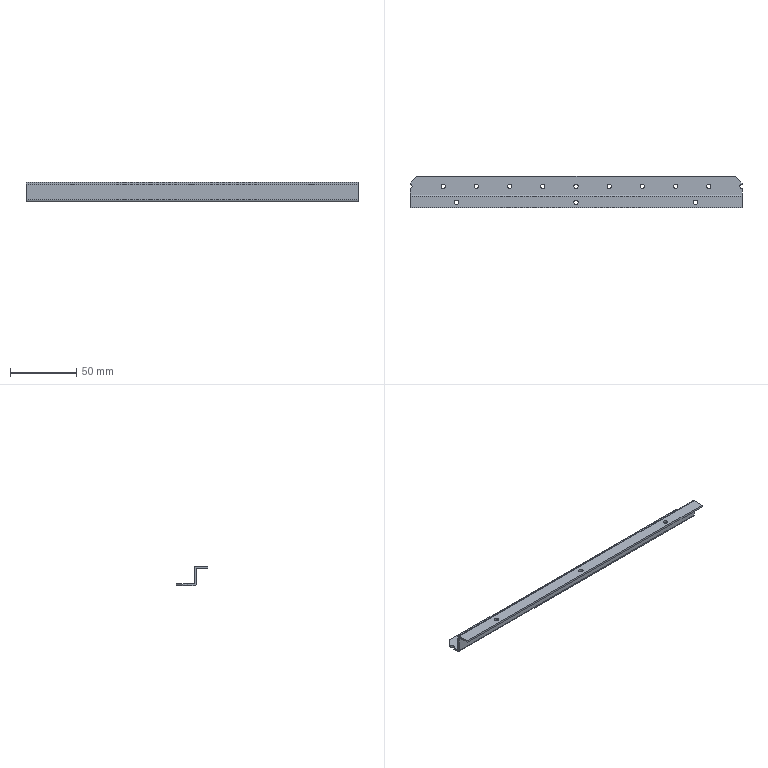Part | SolidWorks | features LPattern 4, EdgeFlange 2, ICE 2, Chamfer 1, FlatPattern 1, SMBaseFlange 1, SheetMetal 1 | 1 solid | 53 faces | box 250 x 23.5 x 15 mm | volume 13407 mm3 | cylinder 31 | plane 22 | commonest cylinder face diameters 3.2 x29 0.2 x2